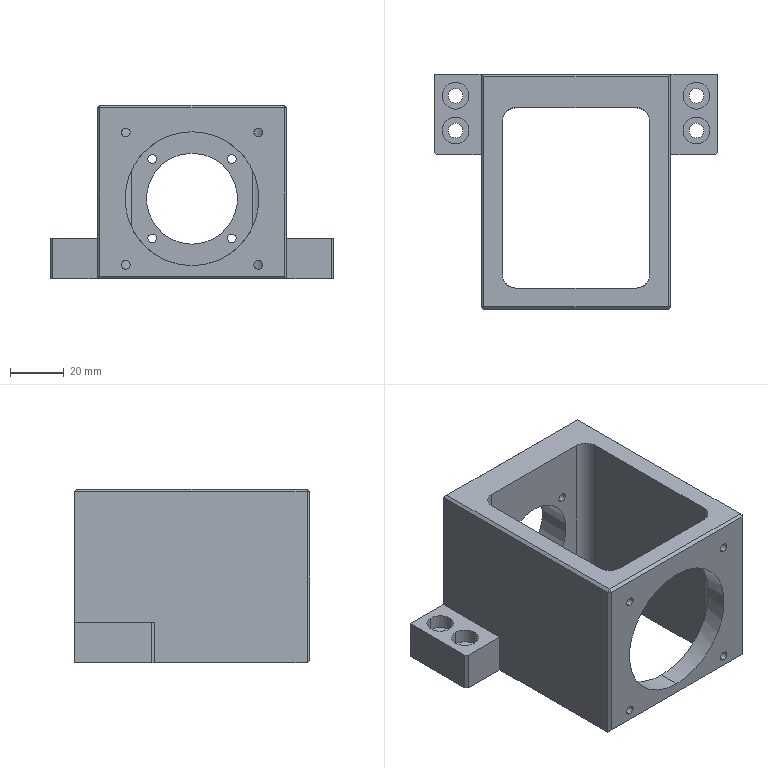CAM job | NX | 3-axis milling, drilling | part box 106 x 88 x 65 mm | stock box 112 x 94 x 66 mm
Tools:
number,name,description,diameter,corner_radius,flute_length,length,flutes
1,D63,Milling Tool-5 Parameters,63.0,0.0,50.0,75.0,2
20,D20,Milling Tool-5 Parameters,20.0,0.0,50.0,75.0,2
11,D10JING,Milling Tool-5 Parameters,10.0,0.0,50.0,75.0,2
7,D6A45,Milling Tool-5 Parameters,6.0,0.0,3.0,3.0,2
15,5.5ZT,Drilling Tool,5.5,0.0,35.0,50.0,2
Operations:
program,operation,operation_type,tool,method,geometry_group,spindle_rpm,surface_speed,feed_per_tooth,feed_cut,feed_plunge,cut_length_mm,path_length_mm,cut_time_min,machine_time_min
1-113-90-70毛胚,FLOOR_WALL,VolumeBased25DMillingOperation,D63,METHOD,A,6500.0,1286.0,0.0962,1250.0,100.0,605.797,659.797,0.4846,0.49
1-113-90-70毛胚,CAVITY_MILL,CavityMilling,D20,METHOD,A,7000.0,439.0,0.1571,2200.0,1000.0,96324.289,123211.918,46.803,49.642
1-113-90-70毛胚,ZLEVEL_PROFILE_COPY_1,ZLevelMilling,D10JING,METHOD,A,7000.0,87.0,0.1071,1500.0,1000.0,9178.622,14221.03,6.662,7.166
1-113-90-70毛胚,ZLEVEL_PROFILE_COPY_COPY_1_1_COPY_COPY,ZLevelMilling,D10JING,METHOD,A,6000.0,188.0,0.0667,800.0,100.0,1096.919,1288.806,1.371,1.39
1-113-90-70毛胚,ZLEVEL_PROFILE_COPY_COPY_1_1_COPY_COPY_COPY_1_COPY,ZLevelMilling,D10JING,METHOD,A,6000.0,188.0,0.0667,800.0,100.0,419.004,577.004,0.5238,0.5396
1-113-90-70毛胚,ZLEVEL_PROFILE_COPY_COPY_1_1_COPY_COPY_COPY_1,ZLevelMilling,D10JING,METHOD,A,6000.0,188.0,0.0667,800.0,100.0,1449.216,1610.187,1.812,1.828
1-113-90-70毛胚,ZLEVEL_PROFILE_COPY_COPY_1_1_COPY_COPY_COPY_1_COPY_1,ZLevelMilling,D10JING,METHOD,A,6000.0,188.0,0.0667,800.0,100.0,426.84,614.84,0.5336,0.5524
1-113-90-70毛胚,DRILLING_COPY_1,Operation,D6A45,METHOD,A,3000.0,56.0,0.0333,200.0,0.0,20.4,326.533,0.102,0.1326
1-113-90-70毛胚,DRILLING_COPY_1_COPY_COPY_1_COPY_1,Operation,5.5ZT,METHOD,A,2000.0,41.0,0.075,300.0,0.0,84.609,454.952,0.282,0.3191
1-113-90-70毛胚,DRILLING_COPY_1_COPY,Operation,D10JING,METHOD,A,2000.0,62.0,0.025,100.0,0.0,33.6,352.933,0.336,0.3679
1-113-90-70毛胚,ZLEVEL_PROFILE_COPY_1_COPY_COPY_COPY_COPY_2_COPY,ZLevelMilling,D6A45,METHOD,A,7000.0,131.0,0.0714,1000.0,1000.0,554.575,753.229,0.5546,0.5744
1-113-90-70毛胚,ZLEVEL_PROFILE_COPY_1_COPY_COPY_COPY_COPY_2_COPY_COPY,ZLevelMilling,D6A45,METHOD,A,7000.0,131.0,0.0714,1000.0,1000.0,245.592,1511.857,0.2456,0.3722